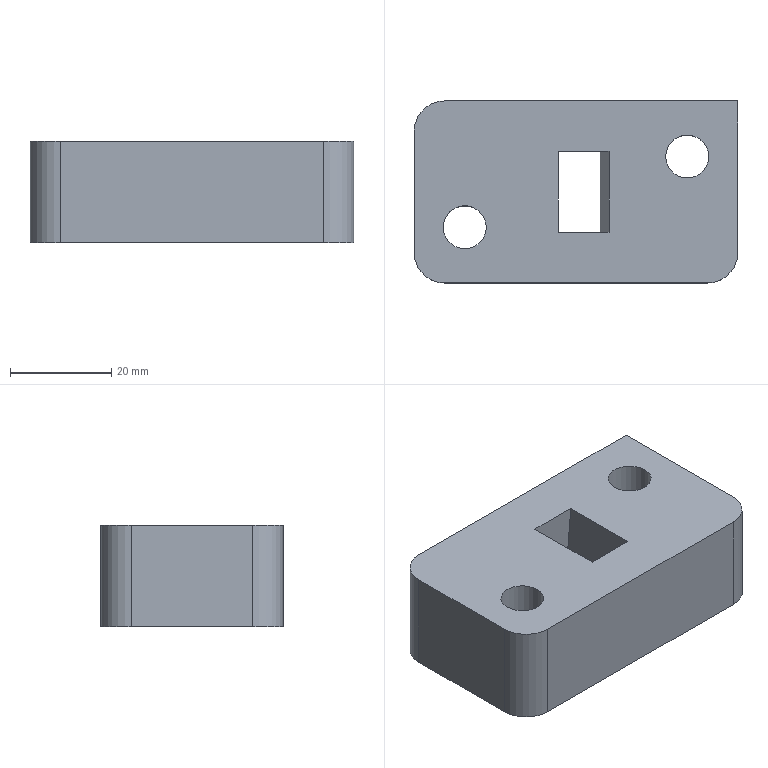Part | STEP file | solid 100 | 1 solid | 36 faces | box 64 x 36 x 20 mm | volume 38384 mm3 | plane 21 | other 8 | cylinder 7 | commonest cylinder face diameters 12 x3 8.5 x2 14 x2